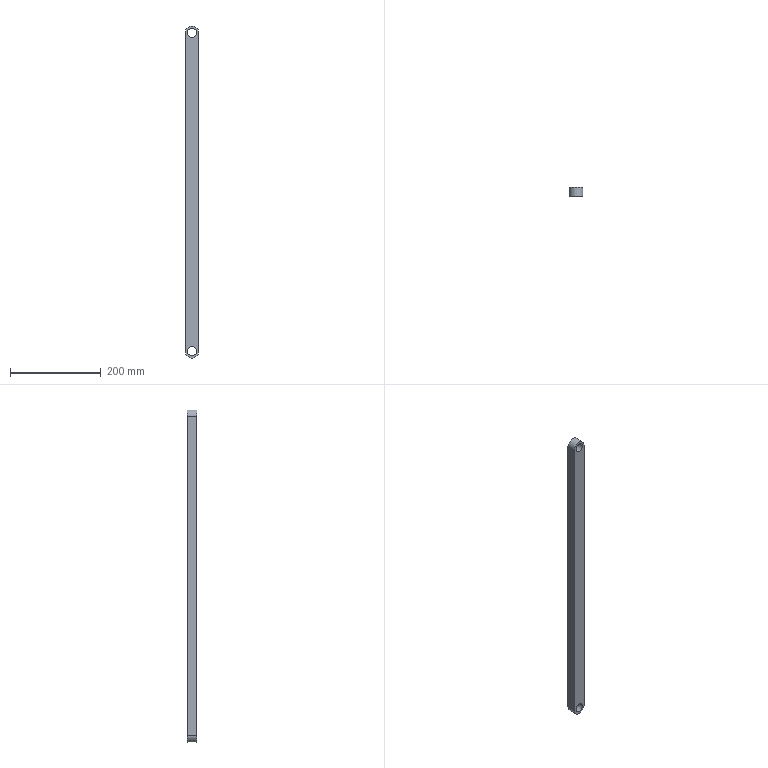Part | SolidWorks | features BaseBody 1 | 1 solid | 22 faces | box 30 x 20 x 730 mm | volume 420440 mm3 | cylinder 14 | plane 8 | commonest cylinder face diameters 6 x8 20 x4 30 x2
STEP:
#1=CARTESIAN_POINT('',(260.959,27.138,-80.));
#2=VERTEX_POINT('',#1);
#3=CARTESIAN_POINT('',(266.959,27.138,-80.));
#4=VERTEX_POINT('',#3);
#5=CARTESIAN_POINT('',(263.959,27.138,-80.));
#6=DIRECTION('',(0.,1.,0.));
#7=DIRECTION('',(-1.,0.,0.));
#8=AXIS2_PLACEMENT_3D('',#5,#6,#7);
#9=CIRCLE('',#8,3.);
#10=EDGE_CURVE('',#2,#4,#9,.T.);
#11=ORIENTED_EDGE('',*,*,#10,.F.);
#12=CARTESIAN_POINT('',(260.959,37.138,-80.));
#13=VERTEX_POINT('',#12);
#14=CARTESIAN_POINT('',(260.959,27.138,-80.));
#15=DIRECTION('',(0.,1.,0.));
#16=VECTOR('',#15,1000.);
#17=LINE('',#14,#16);
#18=EDGE_CURVE('',#2,#13,#17,.T.);
#19=ORIENTED_EDGE('',*,*,#18,.T.);
#20=CARTESIAN_POINT('',(266.959,37.138,-80.));
#21=VERTEX_POINT('',#20);
#22=CARTESIAN_POINT('',(263.959,37.138,-80.));
#23=DIRECTION('',(0.,1.,0.));
#24=DIRECTION('',(-1.,0.,0.));
#25=AXIS2_PLACEMENT_3D('',#22,#23,#24);
#26=CIRCLE('',#25,3.);
#27=EDGE_CURVE('',#13,#21,#26,.T.);
#28=ORIENTED_EDGE('',*,*,#27,.T.);
#29=CARTESIAN_POINT('',(266.959,27.138,-80.));
#30=DIRECTION('',(0.,1.,0.));
#31=VECTOR('',#30,1000.);
#32=LINE('',#29,#31);
#33=EDGE_CURVE('',#4,#21,#32,.T.);
#34=ORIENTED_EDGE('',*,*,#33,.F.);
#35=EDGE_LOOP('',(#11,#19,#28,#34));
#36=FACE_OUTER_BOUND('',#35,.T.);
#37=CARTESIAN_POINT('',(263.959,27.138,-80.));
#38=DIRECTION('',(0.,1.,0.));
#39=DIRECTION('',(1.,0.,0.));
#40=AXIS2_PLACEMENT_3D('',#37,#38,#39);
#41=CYLINDRICAL_SURFACE('',#40,3.);
#42=ADVANCED_FACE('',(#36),#41,.F.);
#43=CARTESIAN_POINT('',(260.959,27.138,-40.));
#44=VERTEX_POINT('',#43);
#45=CARTESIAN_POINT('',(266.959,27.138,-40.));
#46=VERTEX_POINT('',#45);
#47=CARTESIAN_POINT('',(263.959,27.138,-40.));
#48=DIRECTION('',(0.,1.,0.));
#49=DIRECTION('',(-1.,0.,0.));
#50=AXIS2_PLACEMENT_3D('',#47,#48,#49);
#51=CIRCLE('',#50,3.);
#52=EDGE_CURVE('',#44,#46,#51,.T.);
#53=ORIENTED_EDGE('',*,*,#52,.F.);
#54=CARTESIAN_POINT('',(260.959,37.138,-40.));
#55=VERTEX_POINT('',#54);
#56=CARTESIAN_POINT('',(260.959,27.138,-40.));
#57=DIRECTION('',(0.,1.,0.));
#58=VECTOR('',#57,1000.);
#59=LINE('',#56,#58);
#60=EDGE_CURVE('',#44,#55,#59,.T.);
#61=ORIENTED_EDGE('',*,*,#60,.T.);
#62=CARTESIAN_POINT('',(266.959,37.138,-40.));
#63=VERTEX_POINT('',#62);
#64=CARTESIAN_POINT('',(263.959,37.138,-40.));
#65=DIRECTION('',(0.,1.,0.));
#66=DIRECTION('',(-1.,0.,0.));
#67=AXIS2_PLACEMENT_3D('',#64,#65,#66);
#68=CIRCLE('',#67,3.);
#69=EDGE_CURVE('',#55,#63,#68,.T.);
#70=ORIENTED_EDGE('',*,*,#69,.T.);
#71=CARTESIAN_POINT('',(266.959,27.138,-40.));
#72=DIRECTION('',(0.,1.,0.));
#73=VECTOR('',#72,1000.);
#74=LINE('',#71,#73);
#75=EDGE_CURVE('',#46,#63,#74,.T.);
#76=ORIENTED_EDGE('',*,*,#75,.F.);
#77=EDGE_LOOP('',(#53,#61,#70,#76));
#78=FACE_OUTER_BOUND('',#77,.T.);
#79=CARTESIAN_POINT('',(263.959,27.138,-40.));
#80=DIRECTION('',(0.,1.,0.));
#81=DIRECTION('',(1.,0.,0.));
#82=AXIS2_PLACEMENT_3D('',#79,#80,#81);
#83=CYLINDRICAL_SURFACE('',#82,3.);
#84=ADVANCED_FACE('',(#78),#83,.F.);
#85=CARTESIAN_POINT('',(260.959,27.138,80.));
#86=VERTEX_POINT('',#85);
#87=CARTESIAN_POINT('',(266.959,27.138,80.));
#88=VERTEX_POINT('',#87);
#89=CARTESIAN_POINT('',(263.959,27.138,80.));
#90=DIRECTION('',(0.,1.,0.));
#91=DIRECTION('',(1.,0.,0.));
#92=AXIS2_PLACEMENT_3D('',#89,#90,#91);
#93=CIRCLE('',#92,3.);
#94=EDGE_CURVE('',#86,#88,#93,.T.);
#95=ORIENTED_EDGE('',*,*,#94,.F.);
#96=CARTESIAN_POINT('',(260.959,37.138,80.));
#97=VERTEX_POINT('',#96);
#98=CARTESIAN_POINT('',(260.959,27.138,80.));
#99=DIRECTION('',(0.,1.,0.));
#100=VECTOR('',#99,1000.);
#101=LINE('',#98,#100);
#102=EDGE_CURVE('',#86,#97,#101,.T.);
#103=ORIENTED_EDGE('',*,*,#102,.T.);
#104=CARTESIAN_POINT('',(266.959,37.138,80.));
#105=VERTEX_POINT('',#104);
#106=CARTESIAN_POINT('',(263.959,37.138,80.));
#107=DIRECTION('',(0.,1.,0.));
#108=DIRECTION('',(1.,0.,0.));
#109=AXIS2_PLACEMENT_3D('',#106,#107,#108);
#110=CIRCLE('',#109,3.);
#111=EDGE_CURVE('',#97,#105,#110,.T.);
#112=ORIENTED_EDGE('',*,*,#111,.T.);
#113=CARTESIAN_POINT('',(266.959,27.138,80.));
#114=DIRECTION('',(0.,1.,0.));
#115=VECTOR('',#114,1000.);
#116=LINE('',#113,#115);
#117=EDGE_CURVE('',#88,#105,#116,.T.);
#118=ORIENTED_EDGE('',*,*,#117,.F.);
#119=EDGE_LOOP('',(#95,#103,#112,#118));
#120=FACE_OUTER_BOUND('',#119,.T.);
#121=CARTESIAN_POINT('',(263.959,27.138,80.));
#122=DIRECTION('',(0.,1.,0.));
#123=DIRECTION('',(1.,0.,0.));
#124=AXIS2_PLACEMENT_3D('',#121,#122,#123);
#125=CYLINDRICAL_SURFACE('',#124,3.);
#126=ADVANCED_FACE('',(#120),#125,.F.);
#127=CARTESIAN_POINT('',(260.959,27.138,40.));
#128=VERTEX_POINT('',#127);
#129=CARTESIAN_POINT('',(266.959,27.138,40.));
#130=VERTEX_POINT('',#129);
#131=CARTESIAN_POINT('',(263.959,27.138,40.));
#132=DIRECTION('',(0.,1.,0.));
#133=DIRECTION('',(1.,0.,0.));
#134=AXIS2_PLACEMENT_3D('',#131,#132,#133);
#135=CIRCLE('',#134,3.);
#136=EDGE_CURVE('',#128,#130,#135,.T.);
#137=ORIENTED_EDGE('',*,*,#136,.F.);
#138=CARTESIAN_POINT('',(260.959,37.138,40.));
#139=VERTEX_POINT('',#138);
#140=CARTESIAN_POINT('',(260.959,27.138,40.));
#141=DIRECTION('',(0.,1.,0.));
#142=VECTOR('',#141,1000.);
#143=LINE('',#140,#142);
#144=EDGE_CURVE('',#128,#139,#143,.T.);
#145=ORIENTED_EDGE('',*,*,#144,.T.);
#146=CARTESIAN_POINT('',(266.959,37.138,40.));
#147=VERTEX_POINT('',#146);
#148=CARTESIAN_POINT('',(263.959,37.138,40.));
#149=DIRECTION('',(0.,1.,0.));
#150=DIRECTION('',(1.,0.,0.));
#151=AXIS2_PLACEMENT_3D('',#148,#149,#150);
#152=CIRCLE('',#151,3.);
#153=EDGE_CURVE('',#139,#147,#152,.T.);
#154=ORIENTED_EDGE('',*,*,#153,.T.);
#155=CARTESIAN_POINT('',(266.959,27.138,40.));
#156=DIRECTION('',(0.,1.,0.));
#157=VECTOR('',#156,1000.);
#158=LINE('',#155,#157);
#159=EDGE_CURVE('',#130,#147,#158,.T.);
#160=ORIENTED_EDGE('',*,*,#159,.F.);
#161=EDGE_LOOP('',(#137,#145,#154,#160));
#162=FACE_OUTER_BOUND('',#161,.T.);
#163=CARTESIAN_POINT('',(263.959,27.138,40.));
#164=DIRECTION('',(0.,1.,0.));
#165=DIRECTION('',(1.,0.,0.));
#166=AXIS2_PLACEMENT_3D('',#163,#164,#165);
#167=CYLINDRICAL_SURFACE('',#166,3.);
#168=ADVANCED_FACE('',(#162),#167,.F.);
#169=CARTESIAN_POINT('',(258.959,37.138,-350.));
#170=VERTEX_POINT('',#169);
#171=CARTESIAN_POINT('',(278.959,37.138,-350.));
#172=VERTEX_POINT('',#171);
#173=CARTESIAN_POINT('',(268.959,37.138,-350.));
#174=DIRECTION('',(0.,1.,0.));
#175=DIRECTION('',(1.,0.,0.));
#176=AXIS2_PLACEMENT_3D('',#173,#174,#175);
#177=CIRCLE('',#176,10.);
#178=EDGE_CURVE('',#170,#172,#177,.T.);
#179=ORIENTED_EDGE('',*,*,#178,.T.);
#180=CARTESIAN_POINT('',(278.959,17.138,-350.));
#181=VERTEX_POINT('',#180);
#182=CARTESIAN_POINT('',(278.959,37.138,-350.));
#183=DIRECTION('',(0.,-1.,0.));
#184=VECTOR('',#183,1000.);
#185=LINE('',#182,#184);
#186=EDGE_CURVE('',#172,#181,#185,.T.);
#187=ORIENTED_EDGE('',*,*,#186,.T.);
#188=CARTESIAN_POINT('',(258.959,17.138,-350.));
#189=VERTEX_POINT('',#188);
#190=CARTESIAN_POINT('',(268.959,17.138,-350.));
#191=DIRECTION('',(0.,1.,0.));
#192=DIRECTION('',(1.,0.,0.));
#193=AXIS2_PLACEMENT_3D('',#190,#191,#192);
#194=CIRCLE('',#193,10.);
#195=EDGE_CURVE('',#189,#181,#194,.T.);
#196=ORIENTED_EDGE('',*,*,#195,.F.);
#197=CARTESIAN_POINT('',(258.959,37.138,-350.));
#198=DIRECTION('',(0.,-1.,0.));
#199=VECTOR('',#198,1000.);
#200=LINE('',#197,#199);
#201=EDGE_CURVE('',#170,#189,#200,.T.);
#202=ORIENTED_EDGE('',*,*,#201,.F.);
#203=EDGE_LOOP('',(#179,#187,#196,#202));
#204=FACE_OUTER_BOUND('',#203,.T.);
#205=CARTESIAN_POINT('',(268.959,37.138,-350.));
#206=DIRECTION('',(0.,-1.,0.));
#207=DIRECTION('',(-1.,0.,0.));
#208=AXIS2_PLACEMENT_3D('',#205,#206,#207);
#209=CYLINDRICAL_SURFACE('',#208,10.);
#210=ADVANCED_FACE('',(#204),#209,.F.);
#211=CARTESIAN_POINT('',(258.959,37.138,350.));
#212=VERTEX_POINT('',#211);
#213=CARTESIAN_POINT('',(278.959,37.138,350.));
#214=VERTEX_POINT('',#213);
#215=CARTESIAN_POINT('',(268.959,37.138,350.));
#216=DIRECTION('',(0.,1.,0.));
#217=DIRECTION('',(1.,0.,0.));
#218=AXIS2_PLACEMENT_3D('',#215,#216,#217);
#219=CIRCLE('',#218,10.);
#220=EDGE_CURVE('',#212,#214,#219,.T.);
#221=ORIENTED_EDGE('',*,*,#220,.T.);
#222=CARTESIAN_POINT('',(278.959,17.138,350.));
#223=VERTEX_POINT('',#222);
#224=CARTESIAN_POINT('',(278.959,37.138,350.));
#225=DIRECTION('',(0.,-1.,0.));
#226=VECTOR('',#225,1000.);
#227=LINE('',#224,#226);
#228=EDGE_CURVE('',#214,#223,#227,.T.);
#229=ORIENTED_EDGE('',*,*,#228,.T.);
#230=CARTESIAN_POINT('',(258.959,17.138,350.));
#231=VERTEX_POINT('',#230);
#232=CARTESIAN_POINT('',(268.959,17.138,350.));
#233=DIRECTION('',(0.,1.,0.));
#234=DIRECTION('',(1.,0.,0.));
#235=AXIS2_PLACEMENT_3D('',#232,#233,#234);
#236=CIRCLE('',#235,10.);
#237=EDGE_CURVE('',#231,#223,#236,.T.);
#238=ORIENTED_EDGE('',*,*,#237,.F.);
#239=CARTESIAN_POINT('',(258.959,37.138,350.));
#240=DIRECTION('',(0.,-1.,0.));
#241=VECTOR('',#240,1000.);
#242=LINE('',#239,#241);
#243=EDGE_CURVE('',#212,#231,#242,.T.);
#244=ORIENTED_EDGE('',*,*,#243,.F.);
#245=EDGE_LOOP('',(#221,#229,#238,#244));
#246=FACE_OUTER_BOUND('',#245,.T.);
#247=CARTESIAN_POINT('',(268.959,37.138,350.));
#248=DIRECTION('',(0.,-1.,0.));
#249=DIRECTION('',(-1.,0.,0.));
#250=AXIS2_PLACEMENT_3D('',#247,#248,#249);
#251=CYLINDRICAL_SURFACE('',#250,10.);
#252=ADVANCED_FACE('',(#246),#251,.F.);
#253=CARTESIAN_POINT('',(263.959,37.138,-80.));
#254=DIRECTION('',(0.,1.,0.));
#255=DIRECTION('',(-1.,0.,0.));
#256=AXIS2_PLACEMENT_3D('',#253,#254,#255);
#257=CIRCLE('',#256,3.);
#258=EDGE_CURVE('',#21,#13,#257,.T.);
#259=ORIENTED_EDGE('',*,*,#258,.F.);
#260=ORIENTED_EDGE('',*,*,#27,.F.);
#261=EDGE_LOOP('',(#259,#260));
#262=FACE_BOUND('',#261,.T.);
#263=CARTESIAN_POINT('',(263.959,37.138,-40.));
#264=DIRECTION('',(0.,1.,0.));
#265=DIRECTION('',(-1.,0.,0.));
#266=AXIS2_PLACEMENT_3D('',#263,#264,#265);
#267=CIRCLE('',#266,3.);
#268=EDGE_CURVE('',#63,#55,#267,.T.);
#269=ORIENTED_EDGE('',*,*,#268,.F.);
#270=ORIENTED_EDGE('',*,*,#69,.F.);
#271=EDGE_LOOP('',(#269,#270));
#272=FACE_BOUND('',#271,.T.);
#273=CARTESIAN_POINT('',(263.959,37.138,80.));
#274=DIRECTION('',(0.,1.,0.));
#275=DIRECTION('',(1.,0.,0.));
#276=AXIS2_PLACEMENT_3D('',#273,#274,#275);
#277=CIRCLE('',#276,3.);
#278=EDGE_CURVE('',#105,#97,#277,.T.);
#279=ORIENTED_EDGE('',*,*,#278,.F.);
#280=ORIENTED_EDGE('',*,*,#111,.F.);
#281=EDGE_LOOP('',(#279,#280));
#282=FACE_BOUND('',#281,.T.);
#283=CARTESIAN_POINT('',(263.959,37.138,40.));
#284=DIRECTION('',(0.,1.,0.));
#285=DIRECTION('',(1.,0.,0.));
#286=AXIS2_PLACEMENT_3D('',#283,#284,#285);
#287=CIRCLE('',#286,3.);
#288=EDGE_CURVE('',#147,#139,#287,.T.);
#289=ORIENTED_EDGE('',*,*,#288,.F.);
#290=ORIENTED_EDGE('',*,*,#153,.F.);
#291=EDGE_LOOP('',(#289,#290));
#292=FACE_BOUND('',#291,.T.);
#293=ORIENTED_EDGE('',*,*,#220,.F.);
#294=CARTESIAN_POINT('',(268.959,37.138,350.));
#295=DIRECTION('',(0.,1.,0.));
#296=DIRECTION('',(1.,0.,0.));
#297=AXIS2_PLACEMENT_3D('',#294,#295,#296);
#298=CIRCLE('',#297,10.);
#299=EDGE_CURVE('',#214,#212,#298,.T.);
#300=ORIENTED_EDGE('',*,*,#299,.F.);
#301=EDGE_LOOP('',(#293,#300));
#302=FACE_BOUND('',#301,.T.);
#303=CARTESIAN_POINT('',(253.959,37.138,350.));
#304=VERTEX_POINT('',#303);
#305=CARTESIAN_POINT('',(283.959,37.138,350.));
#306=VERTEX_POINT('',#305);
#307=CARTESIAN_POINT('',(268.959,37.138,350.));
#308=DIRECTION('',(0.,1.,0.));
#309=DIRECTION('',(1.,0.,0.));
#310=AXIS2_PLACEMENT_3D('',#307,#308,#309);
#311=CIRCLE('',#310,15.);
#312=EDGE_CURVE('',#304,#306,#311,.T.);
#313=ORIENTED_EDGE('',*,*,#312,.T.);
#314=CARTESIAN_POINT('',(283.959,37.138,-350.));
#315=VERTEX_POINT('',#314);
#316=CARTESIAN_POINT('',(283.959,37.138,350.));
#317=DIRECTION('',(0.,0.,-1.));
#318=VECTOR('',#317,1000.);
#319=LINE('',#316,#318);
#320=EDGE_CURVE('',#306,#315,#319,.T.);
#321=ORIENTED_EDGE('',*,*,#320,.T.);
#322=CARTESIAN_POINT('',(253.959,37.138,-350.));
#323=VERTEX_POINT('',#322);
#324=CARTESIAN_POINT('',(268.959,37.138,-350.));
#325=DIRECTION('',(0.,1.,0.));
#326=DIRECTION('',(1.,0.,0.));
#327=AXIS2_PLACEMENT_3D('',#324,#325,#326);
#328=CIRCLE('',#327,15.);
#329=EDGE_CURVE('',#315,#323,#328,.T.);
#330=ORIENTED_EDGE('',*,*,#329,.T.);
#331=CARTESIAN_POINT('',(253.959,37.138,-350.));
#332=DIRECTION('',(0.,0.,1.));
#333=VECTOR('',#332,1000.);
#334=LINE('',#331,#333);
#335=EDGE_CURVE('',#323,#304,#334,.T.);
#336=ORIENTED_EDGE('',*,*,#335,.T.);
#337=EDGE_LOOP('',(#313,#321,#330,#336));
#338=FACE_OUTER_BOUND('',#337,.T.);
#339=ORIENTED_EDGE('',*,*,#178,.F.);
#340=CARTESIAN_POINT('',(268.959,37.138,-350.));
#341=DIRECTION('',(0.,1.,0.));
#342=DIRECTION('',(1.,0.,0.));
#343=AXIS2_PLACEMENT_3D('',#340,#341,#342);
#344=CIRCLE('',#343,10.);
#345=EDGE_CURVE('',#172,#170,#344,.T.);
#346=ORIENTED_EDGE('',*,*,#345,.F.);
#347=EDGE_LOOP('',(#339,#346));
#348=FACE_BOUND('',#347,.T.);
#349=CARTESIAN_POINT('',(268.959,37.138,350.));
#350=DIRECTION('',(0.,1.,0.));
#351=DIRECTION('',(1.,0.,0.));
#352=AXIS2_PLACEMENT_3D('',#349,#350,#351);
#353=PLANE('',#352);
#354=ADVANCED_FACE('',(#262,#272,#282,#292,#302,#338,#348),#353,.T.);
#355=ORIENTED_EDGE('',*,*,#237,.T.);
#356=CARTESIAN_POINT('',(268.959,17.138,350.));
#357=DIRECTION('',(0.,1.,0.));
#358=DIRECTION('',(1.,0.,0.));
#359=AXIS2_PLACEMENT_3D('',#356,#357,#358);
#360=CIRCLE('',#359,10.);
#361=EDGE_CURVE('',#223,#231,#360,.T.);
#362=ORIENTED_EDGE('',*,*,#361,.T.);
#363=EDGE_LOOP('',(#355,#362));
#364=FACE_BOUND('',#363,.T.);
#365=CARTESIAN_POINT('',(253.959,17.138,350.));
#366=VERTEX_POINT('',#365);
#367=CARTESIAN_POINT('',(283.959,17.138,350.));
#368=VERTEX_POINT('',#367);
#369=CARTESIAN_POINT('',(268.959,17.138,350.));
#370=DIRECTION('',(0.,1.,0.));
#371=DIRECTION('',(1.,0.,0.));
#372=AXIS2_PLACEMENT_3D('',#369,#370,#371);
#373=CIRCLE('',#372,15.);
#374=EDGE_CURVE('',#366,#368,#373,.T.);
#375=ORIENTED_EDGE('',*,*,#374,.F.);
#376=CARTESIAN_POINT('',(253.959,17.138,-350.));
#377=VERTEX_POINT('',#376);
#378=CARTESIAN_POINT('',(253.959,17.138,-350.));
#379=DIRECTION('',(0.,0.,1.));
#380=VECTOR('',#379,1000.);
#381=LINE('',#378,#380);
#382=EDGE_CURVE('',#377,#366,#381,.T.);
#383=ORIENTED_EDGE('',*,*,#382,.F.);
#384=CARTESIAN_POINT('',(283.959,17.138,-350.));
#385=VERTEX_POINT('',#384);
#386=CARTESIAN_POINT('',(268.959,17.138,-350.));
#387=DIRECTION('',(0.,1.,0.));
#388=DIRECTION('',(1.,0.,0.));
#389=AXIS2_PLACEMENT_3D('',#386,#387,#388);
#390=CIRCLE('',#389,15.);
#391=EDGE_CURVE('',#385,#377,#390,.T.);
#392=ORIENTED_EDGE('',*,*,#391,.F.);
#393=CARTESIAN_POINT('',(283.959,17.138,350.));
#394=DIRECTION('',(0.,0.,-1.));
#395=VECTOR('',#394,1000.);
#396=LINE('',#393,#395);
#397=EDGE_CURVE('',#368,#385,#396,.T.);
#398=ORIENTED_EDGE('',*,*,#397,.F.);
#399=EDGE_LOOP('',(#375,#383,#392,#398));
#400=FACE_OUTER_BOUND('',#399,.T.);
#401=ORIENTED_EDGE('',*,*,#195,.T.);
#402=CARTESIAN_POINT('',(268.959,17.138,-350.));
#403=DIRECTION('',(0.,1.,0.));
#404=DIRECTION('',(1.,0.,0.));
#405=AXIS2_PLACEMENT_3D('',#402,#403,#404);
#406=CIRCLE('',#405,10.);
#407=EDGE_CURVE('',#181,#189,#406,.T.);
#408=ORIENTED_EDGE('',*,*,#407,.T.);
#409=EDGE_LOOP('',(#401,#408));
#410=FACE_BOUND('',#409,.T.);
#411=CARTESIAN_POINT('',(268.959,17.138,350.));
#412=DIRECTION('',(0.,1.,0.));
#413=DIRECTION('',(1.,0.,0.));
#414=AXIS2_PLACEMENT_3D('',#411,#412,#413);
#415=PLANE('',#414);
#416=ADVANCED_FACE('',(#364,#400,#410),#415,.F.);
#417=ORIENTED_EDGE('',*,*,#374,.T.);
#418=CARTESIAN_POINT('',(283.959,37.138,350.));
#419=DIRECTION('',(0.,-1.,0.));
#420=VECTOR('',#419,1000.);
#421=LINE('',#418,#420);
#422=EDGE_CURVE('',#306,#368,#421,.T.);
#423=ORIENTED_EDGE('',*,*,#422,.F.);
#424=ORIENTED_EDGE('',*,*,#312,.F.);
#425=CARTESIAN_POINT('',(253.959,37.138,350.));
#426=DIRECTION('',(0.,-1.,0.));
#427=VECTOR('',#426,1000.);
#428=LINE('',#425,#427);
#429=EDGE_CURVE('',#304,#366,#428,.T.);
#430=ORIENTED_EDGE('',*,*,#429,.T.);
#431=EDGE_LOOP('',(#417,#423,#424,#430));
#432=FACE_OUTER_BOUND('',#431,.T.);
#433=CARTESIAN_POINT('',(268.959,37.138,350.));
#434=DIRECTION('',(0.,-1.,0.));
#435=DIRECTION('',(-1.,0.,0.));
#436=AXIS2_PLACEMENT_3D('',#433,#434,#435);
#437=CYLINDRICAL_SURFACE('',#436,15.);
#438=ADVANCED_FACE('',(#432),#437,.T.);
#439=ORIENTED_EDGE('',*,*,#397,.T.);
#440=CARTESIAN_POINT('',(283.959,37.138,-350.));
#441=DIRECTION('',(0.,-1.,0.));
#442=VECTOR('',#441,1000.);
#443=LINE('',#440,#442);
#444=EDGE_CURVE('',#315,#385,#443,.T.);
#445=ORIENTED_EDGE('',*,*,#444,.F.);
#446=ORIENTED_EDGE('',*,*,#320,.F.);
#447=ORIENTED_EDGE('',*,*,#422,.T.);
#448=EDGE_LOOP('',(#439,#445,#446,#447));
#449=FACE_OUTER_BOUND('',#448,.T.);
#450=CARTESIAN_POINT('',(283.959,37.138,350.));
#451=DIRECTION('',(-1.,0.,0.));
#452=DIRECTION('',(0.,0.,1.));
#453=AXIS2_PLACEMENT_3D('',#450,#451,#452);
#454=PLANE('',#453);
#455=ADVANCED_FACE('',(#449),#454,.F.);
#456=ORIENTED_EDGE('',*,*,#391,.T.);
#457=CARTESIAN_POINT('',(253.959,37.138,-350.));
#458=DIRECTION('',(0.,-1.,0.));
#459=VECTOR('',#458,1000.);
#460=LINE('',#457,#459);
#461=EDGE_CURVE('',#323,#377,#460,.T.);
#462=ORIENTED_EDGE('',*,*,#461,.F.);
#463=ORIENTED_EDGE('',*,*,#329,.F.);
#464=ORIENTED_EDGE('',*,*,#444,.T.);
#465=EDGE_LOOP('',(#456,#462,#463,#464));
#466=FACE_OUTER_BOUND('',#465,.T.);
#467=CARTESIAN_POINT('',(268.959,37.138,-350.));
#468=DIRECTION('',(0.,-1.,0.));
#469=DIRECTION('',(-1.,0.,0.));
#470=AXIS2_PLACEMENT_3D('',#467,#468,#469);
#471=CYLINDRICAL_SURFACE('',#470,15.);
#472=ADVANCED_FACE('',(#466),#471,.T.);
#473=ORIENTED_EDGE('',*,*,#382,.T.);
#474=ORIENTED_EDGE('',*,*,#429,.F.);
#475=ORIENTED_EDGE('',*,*,#335,.F.);
#476=ORIENTED_EDGE('',*,*,#461,.T.);
#477=EDGE_LOOP('',(#473,#474,#475,#476));
#478=FACE_OUTER_BOUND('',#477,.T.);
#479=CARTESIAN_POINT('',(253.959,37.138,-350.));
#480=DIRECTION('',(1.,0.,0.));
#481=DIRECTION('',(0.,0.,-1.));
#482=AXIS2_PLACEMENT_3D('',#479,#480,#481);
#483=PLANE('',#482);
#484=ADVANCED_FACE('',(#478),#483,.F.);
#485=ORIENTED_EDGE('',*,*,#228,.F.);
#486=ORIENTED_EDGE('',*,*,#299,.T.);
#487=ORIENTED_EDGE('',*,*,#243,.T.);
#488=ORIENTED_EDGE('',*,*,#361,.F.);
#489=EDGE_LOOP('',(#485,#486,#487,#488));
#490=FACE_OUTER_BOUND('',#489,.T.);
#491=CARTESIAN_POINT('',(268.959,37.138,350.));
#492=DIRECTION('',(0.,-1.,0.));
#493=DIRECTION('',(-1.,0.,0.));
#494=AXIS2_PLACEMENT_3D('',#491,#492,#493);
#495=CYLINDRICAL_SURFACE('',#494,10.);
#496=ADVANCED_FACE('',(#490),#495,.F.);
#497=ORIENTED_EDGE('',*,*,#186,.F.);
#498=ORIENTED_EDGE('',*,*,#345,.T.);
#499=ORIENTED_EDGE('',*,*,#201,.T.);
#500=ORIENTED_EDGE('',*,*,#407,.F.);
#501=EDGE_LOOP('',(#497,#498,#499,#500));
#502=FACE_OUTER_BOUND('',#501,.T.);
#503=CARTESIAN_POINT('',(268.959,37.138,-350.));
#504=DIRECTION('',(0.,-1.,0.));
#505=DIRECTION('',(-1.,0.,0.));
#506=AXIS2_PLACEMENT_3D('',#503,#504,#505);
#507=CYLINDRICAL_SURFACE('',#506,10.);
#508=ADVANCED_FACE('',(#502),#507,.F.);
#509=ORIENTED_EDGE('',*,*,#144,.F.);
#510=CARTESIAN_POINT('',(263.959,27.138,40.));
#511=DIRECTION('',(0.,1.,0.));
#512=DIRECTION('',(1.,0.,0.));
#513=AXIS2_PLACEMENT_3D('',#510,#511,#512);
#514=CIRCLE('',#513,3.);
#515=EDGE_CURVE('',#130,#128,#514,.T.);
#516=ORIENTED_EDGE('',*,*,#515,.F.);
#517=ORIENTED_EDGE('',*,*,#159,.T.);
#518=ORIENTED_EDGE('',*,*,#288,.T.);
#519=EDGE_LOOP('',(#509,#516,#517,#518));
#520=FACE_OUTER_BOUND('',#519,.T.);
#521=CARTESIAN_POINT('',(263.959,27.138,40.));
#522=DIRECTION('',(0.,1.,0.));
#523=DIRECTION('',(1.,0.,0.));
#524=AXIS2_PLACEMENT_3D('',#521,#522,#523);
#525=CYLINDRICAL_SURFACE('',#524,3.);
#526=ADVANCED_FACE('',(#520),#525,.F.);
#527=ORIENTED_EDGE('',*,*,#515,.T.);
#528=ORIENTED_EDGE('',*,*,#136,.T.);
#529=EDGE_LOOP('',(#527,#528));
#530=FACE_OUTER_BOUND('',#529,.T.);
#531=CARTESIAN_POINT('',(263.959,27.138,40.));
#532=DIRECTION('',(0.,1.,0.));
#533=DIRECTION('',(1.,0.,0.));
#534=AXIS2_PLACEMENT_3D('',#531,#532,#533);
#535=PLANE('',#534);
#536=ADVANCED_FACE('',(#530),#535,.T.);
#537=ORIENTED_EDGE('',*,*,#102,.F.);
#538=CARTESIAN_POINT('',(263.959,27.138,80.));
#539=DIRECTION('',(0.,1.,0.));
#540=DIRECTION('',(1.,0.,0.));
#541=AXIS2_PLACEMENT_3D('',#538,#539,#540);
#542=CIRCLE('',#541,3.);
#543=EDGE_CURVE('',#88,#86,#542,.T.);
#544=ORIENTED_EDGE('',*,*,#543,.F.);
#545=ORIENTED_EDGE('',*,*,#117,.T.);
#546=ORIENTED_EDGE('',*,*,#278,.T.);
#547=EDGE_LOOP('',(#537,#544,#545,#546));
#548=FACE_OUTER_BOUND('',#547,.T.);
#549=CARTESIAN_POINT('',(263.959,27.138,80.));
#550=DIRECTION('',(0.,1.,0.));
#551=DIRECTION('',(1.,0.,0.));
#552=AXIS2_PLACEMENT_3D('',#549,#550,#551);
#553=CYLINDRICAL_SURFACE('',#552,3.);
#554=ADVANCED_FACE('',(#548),#553,.F.);
#555=ORIENTED_EDGE('',*,*,#543,.T.);
#556=ORIENTED_EDGE('',*,*,#94,.T.);
#557=EDGE_LOOP('',(#555,#556));
#558=FACE_OUTER_BOUND('',#557,.T.);
#559=CARTESIAN_POINT('',(263.959,27.138,80.));
#560=DIRECTION('',(0.,1.,0.));
#561=DIRECTION('',(1.,0.,0.));
#562=AXIS2_PLACEMENT_3D('',#559,#560,#561);
#563=PLANE('',#562);
#564=ADVANCED_FACE('',(#558),#563,.T.);
#565=ORIENTED_EDGE('',*,*,#60,.F.);
#566=CARTESIAN_POINT('',(263.959,27.138,-40.));
#567=DIRECTION('',(0.,1.,0.));
#568=DIRECTION('',(-1.,0.,0.));
#569=AXIS2_PLACEMENT_3D('',#566,#567,#568);
#570=CIRCLE('',#569,3.);
#571=EDGE_CURVE('',#46,#44,#570,.T.);
#572=ORIENTED_EDGE('',*,*,#571,.F.);
#573=ORIENTED_EDGE('',*,*,#75,.T.);
#574=ORIENTED_EDGE('',*,*,#268,.T.);
#575=EDGE_LOOP('',(#565,#572,#573,#574));
#576=FACE_OUTER_BOUND('',#575,.T.);
#577=CARTESIAN_POINT('',(263.959,27.138,-40.));
#578=DIRECTION('',(0.,1.,0.));
#579=DIRECTION('',(1.,0.,0.));
#580=AXIS2_PLACEMENT_3D('',#577,#578,#579);
#581=CYLINDRICAL_SURFACE('',#580,3.);
#582=ADVANCED_FACE('',(#576),#581,.F.);
#583=ORIENTED_EDGE('',*,*,#571,.T.);
#584=ORIENTED_EDGE('',*,*,#52,.T.);
#585=EDGE_LOOP('',(#583,#584));
#586=FACE_OUTER_BOUND('',#585,.T.);
#587=CARTESIAN_POINT('',(263.959,27.138,-40.));
#588=DIRECTION('',(0.,-1.,0.));
#589=DIRECTION('',(-1.,0.,0.));
#590=AXIS2_PLACEMENT_3D('',#587,#588,#589);
#591=PLANE('',#590);
#592=ADVANCED_FACE('',(#586),#591,.F.);
#593=ORIENTED_EDGE('',*,*,#18,.F.);
#594=CARTESIAN_POINT('',(263.959,27.138,-80.));
#595=DIRECTION('',(0.,1.,0.));
#596=DIRECTION('',(-1.,0.,0.));
#597=AXIS2_PLACEMENT_3D('',#594,#595,#596);
#598=CIRCLE('',#597,3.);
#599=EDGE_CURVE('',#4,#2,#598,.T.);
#600=ORIENTED_EDGE('',*,*,#599,.F.);
#601=ORIENTED_EDGE('',*,*,#33,.T.);
#602=ORIENTED_EDGE('',*,*,#258,.T.);
#603=EDGE_LOOP('',(#593,#600,#601,#602));
#604=FACE_OUTER_BOUND('',#603,.T.);
#605=CARTESIAN_POINT('',(263.959,27.138,-80.));
#606=DIRECTION('',(0.,1.,0.));
#607=DIRECTION('',(1.,0.,0.));
#608=AXIS2_PLACEMENT_3D('',#605,#606,#607);
#609=CYLINDRICAL_SURFACE('',#608,3.);
#610=ADVANCED_FACE('',(#604),#609,.F.);
#611=ORIENTED_EDGE('',*,*,#599,.T.);
#612=ORIENTED_EDGE('',*,*,#10,.T.);
#613=EDGE_LOOP('',(#611,#612));
#614=FACE_OUTER_BOUND('',#613,.T.);
#615=CARTESIAN_POINT('',(263.959,27.138,-80.));
#616=DIRECTION('',(0.,-1.,0.));
#617=DIRECTION('',(-1.,0.,0.));
#618=AXIS2_PLACEMENT_3D('',#615,#616,#617);
#619=PLANE('',#618);
#620=ADVANCED_FACE('',(#614),#619,.F.);
#621=CLOSED_SHELL('',(#42,#84,#126,#168,#210,#252,#354,#416,#438,#455,#472,#484,#496,#508,#526,#536,#554,#564,#582,#592,#610,#620));
#622=MANIFOLD_SOLID_BREP('',#621);
#623=CARTESIAN_POINT('',(0.,0.,0.));
#624=DIRECTION('',(0.,0.,1.));
#625=DIRECTION('',(1.,0.,0.));
#626=AXIS2_PLACEMENT_3D('',#623,#624,#625);
#627=(LENGTH_UNIT()NAMED_UNIT(*)SI_UNIT(.MILLI.,.METRE.));
#628=UNCERTAINTY_MEASURE_WITH_UNIT(LENGTH_MEASURE(0.00001),#627,'','');
#629=(NAMED_UNIT(*)PLANE_ANGLE_UNIT()SI_UNIT($,.RADIAN.));
#630=(NAMED_UNIT(*)SI_UNIT($,.STERADIAN.)SOLID_ANGLE_UNIT());
#631=(GEOMETRIC_REPRESENTATION_CONTEXT(3)GLOBAL_UNCERTAINTY_ASSIGNED_CONTEXT((#628))GLOBAL_UNIT_ASSIGNED_CONTEXT((#627,#629,#630))REPRESENTATION_CONTEXT('',''));
#632=ADVANCED_BREP_SHAPE_REPRESENTATION('',(#622,#626),#631);